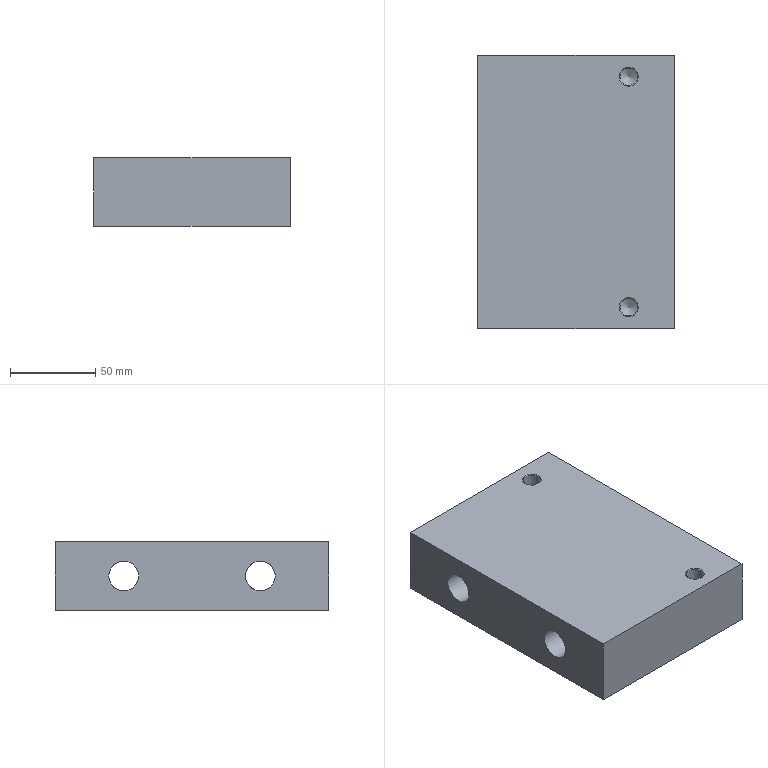Part | STEP file | solid 98 | 1 solid | 18 faces | box 115 x 160 x 40 mm | volume 667851 mm3 | plane 8 | cylinder 6 | cone 4 | commonest cylinder face diameters 10.2 x2 17.5 x2 26 x2